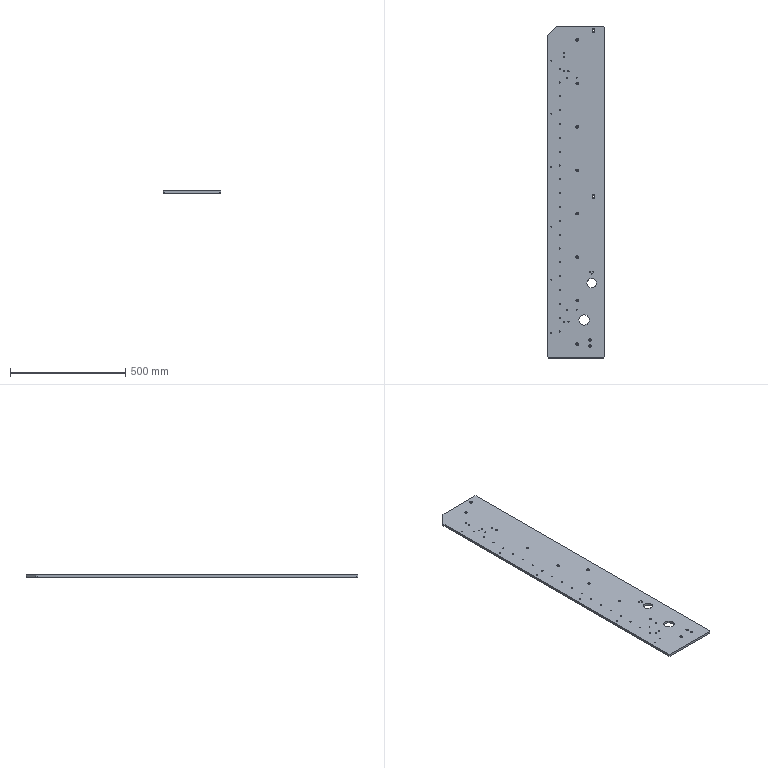Part | SolidWorks | features HoleWzd 9, Cut 2, Chamfer 1, Extrusion 1, Fillet 1 | 1 solid | 162 faces | box 250 x 1440 x 10 mm | volume 3544237 mm3 | cylinder 132 | plane 30 | commonest cylinder face diameters 5 x60 6.6 x24 11 x24 4.2 x14 3.3 x4 20 x2